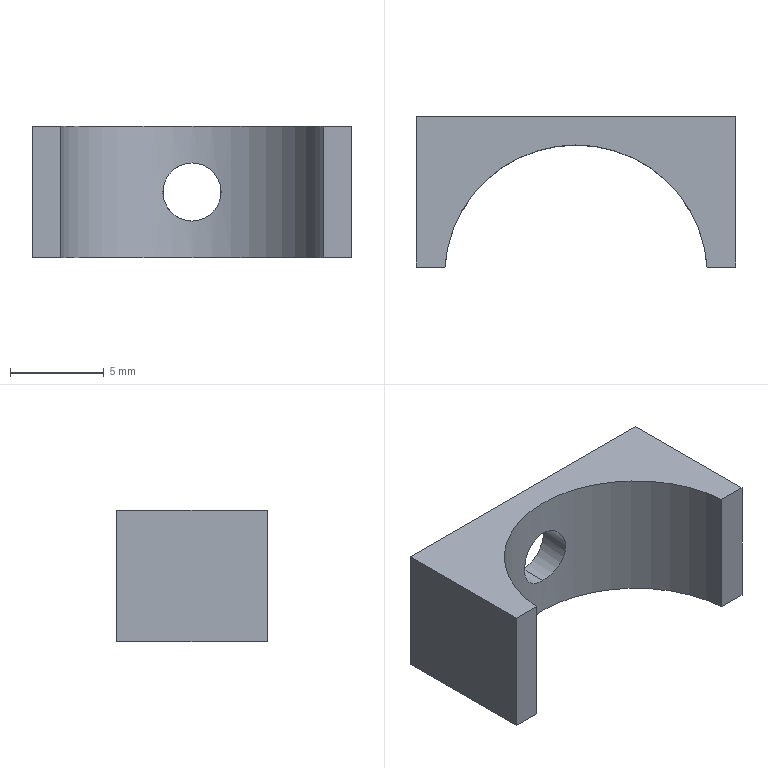Part | SolidWorks | features Extrusion 1, ICE 1 | 1 solid | 10 faces | box 17 x 8 x 7 mm | volume 450.526 mm3 | plane 7 | cylinder 3 | commonest cylinder face diameters 3.1 x2 14 x1
STEP:
#1=CARTESIAN_POINT('',(0.,7.,5.05));
#2=VERTEX_POINT('',#1);
#3=CARTESIAN_POINT('',(0.,7.,1.95));
#4=VERTEX_POINT('',#3);
#5=CARTESIAN_POINT('',(0.,7.,5.05));
#6=CARTESIAN_POINT('',(-0.1028,7.,5.05));
#7=CARTESIAN_POINT('',(-0.2037,6.998,5.04));
#8=CARTESIAN_POINT('',(-0.4023,6.989,5.));
#9=CARTESIAN_POINT('',(-0.5009,6.983,4.97));
#10=CARTESIAN_POINT('',(-0.6885,6.967,4.892));
#11=CARTESIAN_POINT('',(-0.7774,6.957,4.845));
#12=CARTESIAN_POINT('',(-0.9457,6.936,4.732));
#13=CARTESIAN_POINT('',(-1.025,6.925,4.667));
#14=CARTESIAN_POINT('',(-1.239,6.891,4.453));
#15=CARTESIAN_POINT('',(-1.354,6.868,4.281));
#16=CARTESIAN_POINT('',(-1.509,6.836,3.908));
#17=CARTESIAN_POINT('',(-1.55,6.826,3.704));
#18=CARTESIAN_POINT('',(-1.55,6.826,3.399));
#19=CARTESIAN_POINT('',(-1.54,6.829,3.296));
#20=CARTESIAN_POINT('',(-1.5,6.837,3.097));
#21=CARTESIAN_POINT('',(-1.471,6.844,3.));
#22=CARTESIAN_POINT('',(-1.354,6.868,2.718));
#23=CARTESIAN_POINT('',(-1.24,6.891,2.548));
#24=CARTESIAN_POINT('',(-1.024,6.925,2.332));
#25=CARTESIAN_POINT('',(-0.946,6.936,2.268));
#26=CARTESIAN_POINT('',(-0.7784,6.957,2.156));
#27=CARTESIAN_POINT('',(-0.6876,6.967,2.107));
#28=CARTESIAN_POINT('',(-0.5003,6.983,2.029));
#29=CARTESIAN_POINT('',(-0.4036,6.989,2.));
#30=CARTESIAN_POINT('',(-0.2042,6.998,1.96));
#31=CARTESIAN_POINT('',(-0.1013,7.,1.95));
#32=CARTESIAN_POINT('',(0.,7.,1.95));
#33=B_SPLINE_CURVE_WITH_KNOTS('',3,(#5,#6,#7,#8,#9,#10,#11,#12,#13,#14,#15,#16,#17,#18,#19,#20,#21,#22,#23,#24,#25,#26,#27,#28,#29,#30,#31,#32),.UNSPECIFIED.,.F.,.F.,(4,2,2,2,2,2,2,2,2,2,2,2,2,4),(0.,0.0003038,0.0006076,0.0009115,0.001215,0.001823,0.002431,0.002734,0.003038,0.003646,0.00395,0.004253,0.004557,0.004861),.UNSPECIFIED.);
#34=EDGE_CURVE('',#2,#4,#33,.T.);
#35=ORIENTED_EDGE('',*,*,#34,.T.);
#36=CARTESIAN_POINT('',(0.,8.5,1.95));
#37=VERTEX_POINT('',#36);
#38=CARTESIAN_POINT('',(0.,1.5,1.95));
#39=DIRECTION('',(0.,1.,0.));
#40=VECTOR('',#39,1000.);
#41=LINE('',#38,#40);
#42=EDGE_CURVE('',#4,#37,#41,.T.);
#43=ORIENTED_EDGE('',*,*,#42,.T.);
#44=CARTESIAN_POINT('',(0.,8.5,5.05));
#45=VERTEX_POINT('',#44);
#46=CARTESIAN_POINT('',(0.,8.5,3.5));
#47=DIRECTION('',(0.,1.,0.));
#48=DIRECTION('',(0.,0.,1.));
#49=AXIS2_PLACEMENT_3D('',#46,#47,#48);
#50=CIRCLE('',#49,1.55);
#51=EDGE_CURVE('',#37,#45,#50,.T.);
#52=ORIENTED_EDGE('',*,*,#51,.T.);
#53=CARTESIAN_POINT('',(0.,1.5,5.05));
#54=DIRECTION('',(0.,1.,0.));
#55=VECTOR('',#54,1000.);
#56=LINE('',#53,#55);
#57=EDGE_CURVE('',#2,#45,#56,.T.);
#58=ORIENTED_EDGE('',*,*,#57,.F.);
#59=EDGE_LOOP('',(#35,#43,#52,#58));
#60=FACE_OUTER_BOUND('',#59,.T.);
#61=CARTESIAN_POINT('',(0.,1.5,3.5));
#62=DIRECTION('',(0.,1.,0.));
#63=DIRECTION('',(0.,0.,1.));
#64=AXIS2_PLACEMENT_3D('',#61,#62,#63);
#65=CYLINDRICAL_SURFACE('',#64,1.55);
#66=ADVANCED_FACE('',(#60),#65,.F.);
#67=ORIENTED_EDGE('',*,*,#34,.F.);
#68=CARTESIAN_POINT('',(0.,7.,1.95));
#69=CARTESIAN_POINT('',(0.2026,7.,1.95));
#70=CARTESIAN_POINT('',(0.4072,6.991,1.991));
#71=CARTESIAN_POINT('',(0.6871,6.967,2.107));
#72=CARTESIAN_POINT('',(0.7777,6.957,2.155));
#73=CARTESIAN_POINT('',(0.9462,6.936,2.268));
#74=CARTESIAN_POINT('',(1.024,6.925,2.332));
#75=CARTESIAN_POINT('',(1.167,6.902,2.475));
#76=CARTESIAN_POINT('',(1.232,6.891,2.554));
#77=CARTESIAN_POINT('',(1.344,6.87,2.722));
#78=CARTESIAN_POINT('',(1.392,6.86,2.811));
#79=CARTESIAN_POINT('',(1.509,6.836,3.093));
#80=CARTESIAN_POINT('',(1.55,6.826,3.295));
#81=CARTESIAN_POINT('',(1.55,6.826,3.602));
#82=CARTESIAN_POINT('',(1.54,6.829,3.702));
#83=CARTESIAN_POINT('',(1.501,6.837,3.901));
#84=CARTESIAN_POINT('',(1.471,6.844,4.));
#85=CARTESIAN_POINT('',(1.354,6.868,4.281));
#86=CARTESIAN_POINT('',(1.239,6.891,4.453));
#87=CARTESIAN_POINT('',(0.9544,6.936,4.738));
#88=CARTESIAN_POINT('',(0.7822,6.959,4.853));
#89=CARTESIAN_POINT('',(0.5025,6.983,4.97));
#90=CARTESIAN_POINT('',(0.404,6.989,5.));
#91=CARTESIAN_POINT('',(0.2041,6.998,5.04));
#92=CARTESIAN_POINT('',(0.1027,7.,5.05));
#93=CARTESIAN_POINT('',(0.,7.,5.05));
#94=B_SPLINE_CURVE_WITH_KNOTS('',3,(#68,#69,#70,#71,#72,#73,#74,#75,#76,#77,#78,#79,#80,#81,#82,#83,#84,#85,#86,#87,#88,#89,#90,#91,#92,#93),.UNSPECIFIED.,.F.,.F.,(4,2,2,2,2,2,2,2,2,2,2,2,4),(0.004861,0.005469,0.005772,0.006076,0.00638,0.006684,0.007291,0.007595,0.007898,0.008506,0.009113,0.009417,0.009721),.UNSPECIFIED.);
#95=EDGE_CURVE('',#4,#2,#94,.T.);
#96=ORIENTED_EDGE('',*,*,#95,.F.);
#97=EDGE_LOOP('',(#67,#96));
#98=FACE_BOUND('',#97,.T.);
#99=CARTESIAN_POINT('',(6.982,0.5,0.));
#100=VERTEX_POINT('',#99);
#101=CARTESIAN_POINT('',(-6.982,0.5,0.));
#102=VERTEX_POINT('',#101);
#103=CARTESIAN_POINT('',(0.,0.,0.));
#104=DIRECTION('',(0.,0.,1.));
#105=DIRECTION('',(1.,0.,0.));
#106=AXIS2_PLACEMENT_3D('',#103,#104,#105);
#107=CIRCLE('',#106,7.);
#108=EDGE_CURVE('',#100,#102,#107,.T.);
#109=ORIENTED_EDGE('',*,*,#108,.F.);
#110=CARTESIAN_POINT('',(6.982,0.5,7.));
#111=VERTEX_POINT('',#110);
#112=CARTESIAN_POINT('',(6.982,0.5,7.));
#113=DIRECTION('',(0.,0.,-1.));
#114=VECTOR('',#113,1000.);
#115=LINE('',#112,#114);
#116=EDGE_CURVE('',#111,#100,#115,.T.);
#117=ORIENTED_EDGE('',*,*,#116,.F.);
#118=CARTESIAN_POINT('',(-6.982,0.5,7.));
#119=VERTEX_POINT('',#118);
#120=CARTESIAN_POINT('',(0.,0.,7.));
#121=DIRECTION('',(0.,0.,1.));
#122=DIRECTION('',(1.,0.,0.));
#123=AXIS2_PLACEMENT_3D('',#120,#121,#122);
#124=CIRCLE('',#123,7.);
#125=EDGE_CURVE('',#111,#119,#124,.T.);
#126=ORIENTED_EDGE('',*,*,#125,.T.);
#127=CARTESIAN_POINT('',(-6.982,0.5,7.));
#128=DIRECTION('',(0.,0.,-1.));
#129=VECTOR('',#128,1000.);
#130=LINE('',#127,#129);
#131=EDGE_CURVE('',#119,#102,#130,.T.);
#132=ORIENTED_EDGE('',*,*,#131,.T.);
#133=EDGE_LOOP('',(#109,#117,#126,#132));
#134=FACE_OUTER_BOUND('',#133,.T.);
#135=CARTESIAN_POINT('',(0.,0.,7.));
#136=DIRECTION('',(0.,0.,-1.));
#137=DIRECTION('',(-1.,0.,0.));
#138=AXIS2_PLACEMENT_3D('',#135,#136,#137);
#139=CYLINDRICAL_SURFACE('',#138,7.);
#140=ADVANCED_FACE('',(#98,#134),#139,.F.);
#141=CARTESIAN_POINT('',(8.5,0.5,0.));
#142=VERTEX_POINT('',#141);
#143=CARTESIAN_POINT('',(0.,0.5,0.));
#144=DIRECTION('',(1.,0.,0.));
#145=VECTOR('',#144,1000.);
#146=LINE('',#143,#145);
#147=EDGE_CURVE('',#100,#142,#146,.T.);
#148=ORIENTED_EDGE('',*,*,#147,.T.);
#149=CARTESIAN_POINT('',(8.5,0.5,7.));
#150=VERTEX_POINT('',#149);
#151=CARTESIAN_POINT('',(8.5,0.5,7.));
#152=DIRECTION('',(0.,0.,-1.));
#153=VECTOR('',#152,1000.);
#154=LINE('',#151,#153);
#155=EDGE_CURVE('',#150,#142,#154,.T.);
#156=ORIENTED_EDGE('',*,*,#155,.F.);
#157=CARTESIAN_POINT('',(0.,0.5,7.));
#158=DIRECTION('',(1.,0.,0.));
#159=VECTOR('',#158,1000.);
#160=LINE('',#157,#159);
#161=EDGE_CURVE('',#111,#150,#160,.T.);
#162=ORIENTED_EDGE('',*,*,#161,.F.);
#163=ORIENTED_EDGE('',*,*,#116,.T.);
#164=EDGE_LOOP('',(#148,#156,#162,#163));
#165=FACE_OUTER_BOUND('',#164,.T.);
#166=CARTESIAN_POINT('',(0.,0.5,7.));
#167=DIRECTION('',(0.,1.,0.));
#168=DIRECTION('',(0.,0.,1.));
#169=AXIS2_PLACEMENT_3D('',#166,#167,#168);
#170=PLANE('',#169);
#171=ADVANCED_FACE('',(#165),#170,.F.);
#172=CARTESIAN_POINT('',(8.5,8.5,0.));
#173=VERTEX_POINT('',#172);
#174=CARTESIAN_POINT('',(8.5,0.,0.));
#175=DIRECTION('',(0.,-1.,0.));
#176=VECTOR('',#175,1000.);
#177=LINE('',#174,#176);
#178=EDGE_CURVE('',#173,#142,#177,.T.);
#179=ORIENTED_EDGE('',*,*,#178,.F.);
#180=CARTESIAN_POINT('',(8.5,8.5,7.));
#181=VERTEX_POINT('',#180);
#182=CARTESIAN_POINT('',(8.5,8.5,7.));
#183=DIRECTION('',(0.,0.,-1.));
#184=VECTOR('',#183,1000.);
#185=LINE('',#182,#184);
#186=EDGE_CURVE('',#181,#173,#185,.T.);
#187=ORIENTED_EDGE('',*,*,#186,.F.);
#188=CARTESIAN_POINT('',(8.5,0.,7.));
#189=DIRECTION('',(0.,-1.,0.));
#190=VECTOR('',#189,1000.);
#191=LINE('',#188,#190);
#192=EDGE_CURVE('',#181,#150,#191,.T.);
#193=ORIENTED_EDGE('',*,*,#192,.T.);
#194=ORIENTED_EDGE('',*,*,#155,.T.);
#195=EDGE_LOOP('',(#179,#187,#193,#194));
#196=FACE_OUTER_BOUND('',#195,.T.);
#197=CARTESIAN_POINT('',(8.5,0.,7.));
#198=DIRECTION('',(1.,0.,0.));
#199=DIRECTION('',(0.,0.,-1.));
#200=AXIS2_PLACEMENT_3D('',#197,#198,#199);
#201=PLANE('',#200);
#202=ADVANCED_FACE('',(#196),#201,.T.);
#203=CARTESIAN_POINT('',(0.,8.5,3.5));
#204=DIRECTION('',(0.,1.,0.));
#205=DIRECTION('',(0.,0.,1.));
#206=AXIS2_PLACEMENT_3D('',#203,#204,#205);
#207=CIRCLE('',#206,1.55);
#208=EDGE_CURVE('',#45,#37,#207,.T.);
#209=ORIENTED_EDGE('',*,*,#208,.F.);
#210=ORIENTED_EDGE('',*,*,#51,.F.);
#211=EDGE_LOOP('',(#209,#210));
#212=FACE_BOUND('',#211,.T.);
#213=CARTESIAN_POINT('',(-8.5,8.5,0.));
#214=VERTEX_POINT('',#213);
#215=CARTESIAN_POINT('',(0.,8.5,0.));
#216=DIRECTION('',(1.,0.,0.));
#217=VECTOR('',#216,1000.);
#218=LINE('',#215,#217);
#219=EDGE_CURVE('',#214,#173,#218,.T.);
#220=ORIENTED_EDGE('',*,*,#219,.F.);
#221=CARTESIAN_POINT('',(-8.5,8.5,7.));
#222=VERTEX_POINT('',#221);
#223=CARTESIAN_POINT('',(-8.5,8.5,7.));
#224=DIRECTION('',(0.,0.,-1.));
#225=VECTOR('',#224,1000.);
#226=LINE('',#223,#225);
#227=EDGE_CURVE('',#222,#214,#226,.T.);
#228=ORIENTED_EDGE('',*,*,#227,.F.);
#229=CARTESIAN_POINT('',(0.,8.5,7.));
#230=DIRECTION('',(1.,0.,0.));
#231=VECTOR('',#230,1000.);
#232=LINE('',#229,#231);
#233=EDGE_CURVE('',#222,#181,#232,.T.);
#234=ORIENTED_EDGE('',*,*,#233,.T.);
#235=ORIENTED_EDGE('',*,*,#186,.T.);
#236=EDGE_LOOP('',(#220,#228,#234,#235));
#237=FACE_OUTER_BOUND('',#236,.T.);
#238=CARTESIAN_POINT('',(0.,8.5,7.));
#239=DIRECTION('',(0.,1.,0.));
#240=DIRECTION('',(0.,0.,1.));
#241=AXIS2_PLACEMENT_3D('',#238,#239,#240);
#242=PLANE('',#241);
#243=ADVANCED_FACE('',(#212,#237),#242,.T.);
#244=CARTESIAN_POINT('',(-8.5,0.5,0.));
#245=VERTEX_POINT('',#244);
#246=CARTESIAN_POINT('',(-8.5,0.,0.));
#247=DIRECTION('',(0.,-1.,0.));
#248=VECTOR('',#247,1000.);
#249=LINE('',#246,#248);
#250=EDGE_CURVE('',#214,#245,#249,.T.);
#251=ORIENTED_EDGE('',*,*,#250,.T.);
#252=CARTESIAN_POINT('',(-8.5,0.5,7.));
#253=VERTEX_POINT('',#252);
#254=CARTESIAN_POINT('',(-8.5,0.5,7.));
#255=DIRECTION('',(0.,0.,-1.));
#256=VECTOR('',#255,1000.);
#257=LINE('',#254,#256);
#258=EDGE_CURVE('',#253,#245,#257,.T.);
#259=ORIENTED_EDGE('',*,*,#258,.F.);
#260=CARTESIAN_POINT('',(-8.5,0.,7.));
#261=DIRECTION('',(0.,-1.,0.));
#262=VECTOR('',#261,1000.);
#263=LINE('',#260,#262);
#264=EDGE_CURVE('',#222,#253,#263,.T.);
#265=ORIENTED_EDGE('',*,*,#264,.F.);
#266=ORIENTED_EDGE('',*,*,#227,.T.);
#267=EDGE_LOOP('',(#251,#259,#265,#266));
#268=FACE_OUTER_BOUND('',#267,.T.);
#269=CARTESIAN_POINT('',(-8.5,0.,7.));
#270=DIRECTION('',(1.,0.,0.));
#271=DIRECTION('',(0.,0.,-1.));
#272=AXIS2_PLACEMENT_3D('',#269,#270,#271);
#273=PLANE('',#272);
#274=ADVANCED_FACE('',(#268),#273,.F.);
#275=CARTESIAN_POINT('',(0.,0.5,0.));
#276=DIRECTION('',(1.,0.,0.));
#277=VECTOR('',#276,1000.);
#278=LINE('',#275,#277);
#279=EDGE_CURVE('',#245,#102,#278,.T.);
#280=ORIENTED_EDGE('',*,*,#279,.T.);
#281=ORIENTED_EDGE('',*,*,#131,.F.);
#282=CARTESIAN_POINT('',(0.,0.5,7.));
#283=DIRECTION('',(1.,0.,0.));
#284=VECTOR('',#283,1000.);
#285=LINE('',#282,#284);
#286=EDGE_CURVE('',#253,#119,#285,.T.);
#287=ORIENTED_EDGE('',*,*,#286,.F.);
#288=ORIENTED_EDGE('',*,*,#258,.T.);
#289=EDGE_LOOP('',(#280,#281,#287,#288));
#290=FACE_OUTER_BOUND('',#289,.T.);
#291=CARTESIAN_POINT('',(0.,0.5,7.));
#292=DIRECTION('',(0.,1.,0.));
#293=DIRECTION('',(0.,0.,1.));
#294=AXIS2_PLACEMENT_3D('',#291,#292,#293);
#295=PLANE('',#294);
#296=ADVANCED_FACE('',(#290),#295,.F.);
#297=ORIENTED_EDGE('',*,*,#125,.F.);
#298=ORIENTED_EDGE('',*,*,#161,.T.);
#299=ORIENTED_EDGE('',*,*,#192,.F.);
#300=ORIENTED_EDGE('',*,*,#233,.F.);
#301=ORIENTED_EDGE('',*,*,#264,.T.);
#302=ORIENTED_EDGE('',*,*,#286,.T.);
#303=EDGE_LOOP('',(#297,#298,#299,#300,#301,#302));
#304=FACE_OUTER_BOUND('',#303,.T.);
#305=CARTESIAN_POINT('',(0.,0.,7.));
#306=DIRECTION('',(0.,0.,1.));
#307=DIRECTION('',(1.,0.,0.));
#308=AXIS2_PLACEMENT_3D('',#305,#306,#307);
#309=PLANE('',#308);
#310=ADVANCED_FACE('',(#304),#309,.T.);
#311=ORIENTED_EDGE('',*,*,#108,.T.);
#312=ORIENTED_EDGE('',*,*,#279,.F.);
#313=ORIENTED_EDGE('',*,*,#250,.F.);
#314=ORIENTED_EDGE('',*,*,#219,.T.);
#315=ORIENTED_EDGE('',*,*,#178,.T.);
#316=ORIENTED_EDGE('',*,*,#147,.F.);
#317=EDGE_LOOP('',(#311,#312,#313,#314,#315,#316));
#318=FACE_OUTER_BOUND('',#317,.T.);
#319=CARTESIAN_POINT('',(0.,0.,0.));
#320=DIRECTION('',(0.,0.,1.));
#321=DIRECTION('',(1.,0.,0.));
#322=AXIS2_PLACEMENT_3D('',#319,#320,#321);
#323=PLANE('',#322);
#324=ADVANCED_FACE('',(#318),#323,.F.);
#325=ORIENTED_EDGE('',*,*,#42,.F.);
#326=ORIENTED_EDGE('',*,*,#95,.T.);
#327=ORIENTED_EDGE('',*,*,#57,.T.);
#328=ORIENTED_EDGE('',*,*,#208,.T.);
#329=EDGE_LOOP('',(#325,#326,#327,#328));
#330=FACE_OUTER_BOUND('',#329,.T.);
#331=CARTESIAN_POINT('',(0.,1.5,3.5));
#332=DIRECTION('',(0.,1.,0.));
#333=DIRECTION('',(0.,0.,1.));
#334=AXIS2_PLACEMENT_3D('',#331,#332,#333);
#335=CYLINDRICAL_SURFACE('',#334,1.55);
#336=ADVANCED_FACE('',(#330),#335,.F.);
#337=CLOSED_SHELL('',(#66,#140,#171,#202,#243,#274,#296,#310,#324,#336));
#338=MANIFOLD_SOLID_BREP('',#337);
#339=CARTESIAN_POINT('',(0.,0.,0.));
#340=DIRECTION('',(0.,0.,1.));
#341=DIRECTION('',(1.,0.,0.));
#342=AXIS2_PLACEMENT_3D('',#339,#340,#341);
#343=(LENGTH_UNIT()NAMED_UNIT(*)SI_UNIT(.MILLI.,.METRE.));
#344=UNCERTAINTY_MEASURE_WITH_UNIT(LENGTH_MEASURE(0.00001),#343,'','');
#345=(NAMED_UNIT(*)PLANE_ANGLE_UNIT()SI_UNIT($,.RADIAN.));
#346=(NAMED_UNIT(*)SI_UNIT($,.STERADIAN.)SOLID_ANGLE_UNIT());
#347=(GEOMETRIC_REPRESENTATION_CONTEXT(3)GLOBAL_UNCERTAINTY_ASSIGNED_CONTEXT((#344))GLOBAL_UNIT_ASSIGNED_CONTEXT((#343,#345,#346))REPRESENTATION_CONTEXT('',''));
#348=ADVANCED_BREP_SHAPE_REPRESENTATION('',(#338,#342),#347);